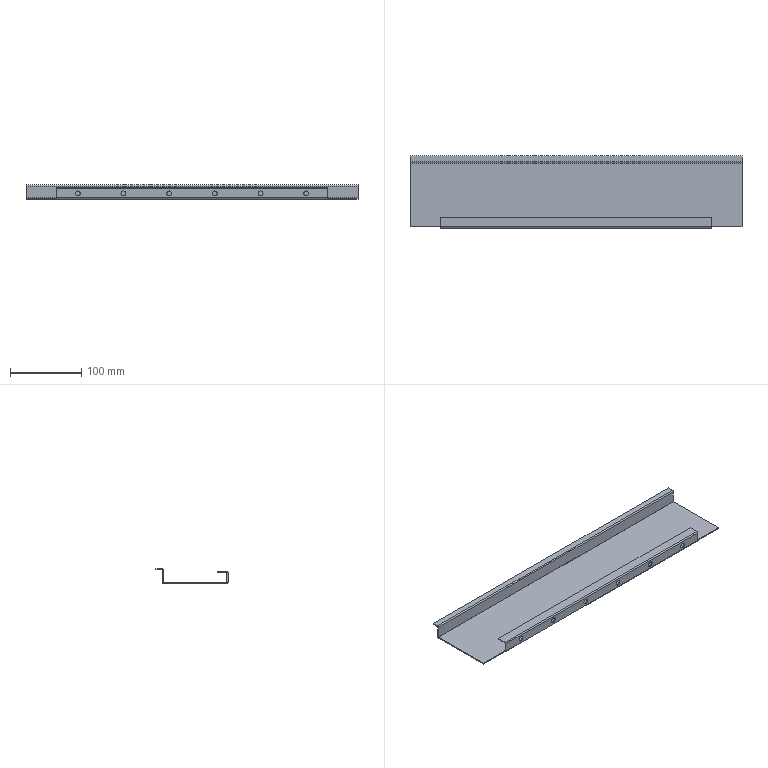Part | STEP file | HESS-408-70-15W-W-35-upper door glass inner frame 1 | 1 solid | 42 faces | box 465 x 101 x 20 mm | volume 97847 mm3 | plane 22 | cylinder 20 | commonest cylinder face diameters 7 x12 0.2 x4 3.2 x4